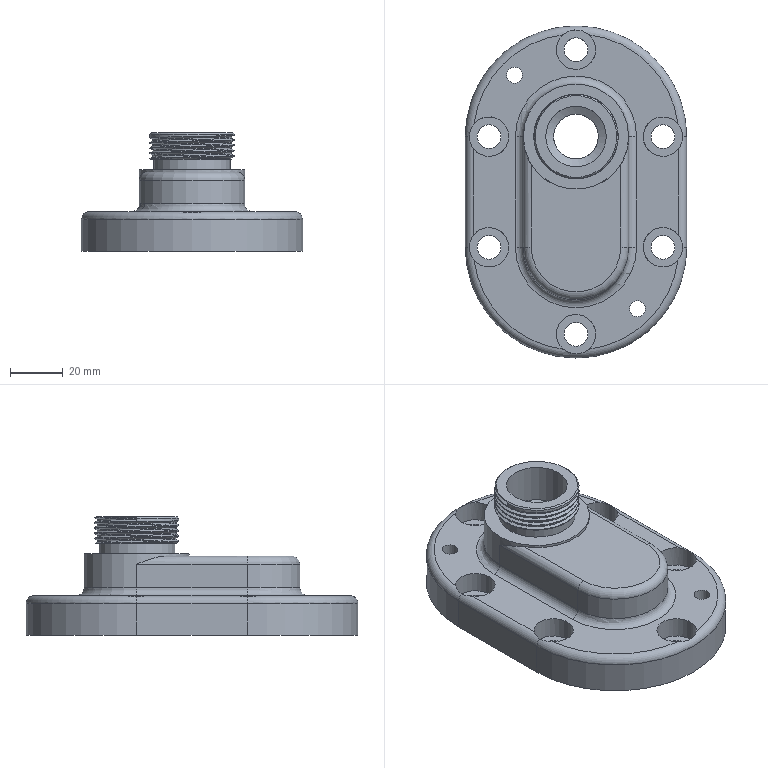Part | NX | features DATUM_CSYS 7, EXTRUDE 7, DATUM_PLANE 6, SKETCH 6, EXTRACT_STRING 2, SWP104 2, BLEND 1, CHAMFER 1, HOLE PACKAGE 1, Instance Feature 1, Mirror Feature 1, SIMPLE HOLE 1, THREADS 1 | 1 solid | 61 faces | box 84 x 126 x 45 mm | volume 154692 mm3 | cylinder 31 | plane 19 | torus 5 | cone 4 | spline 2 | commonest cylinder face diameters 6 x8 9 x6 15 x6 22 x2 40 x2 84 x2